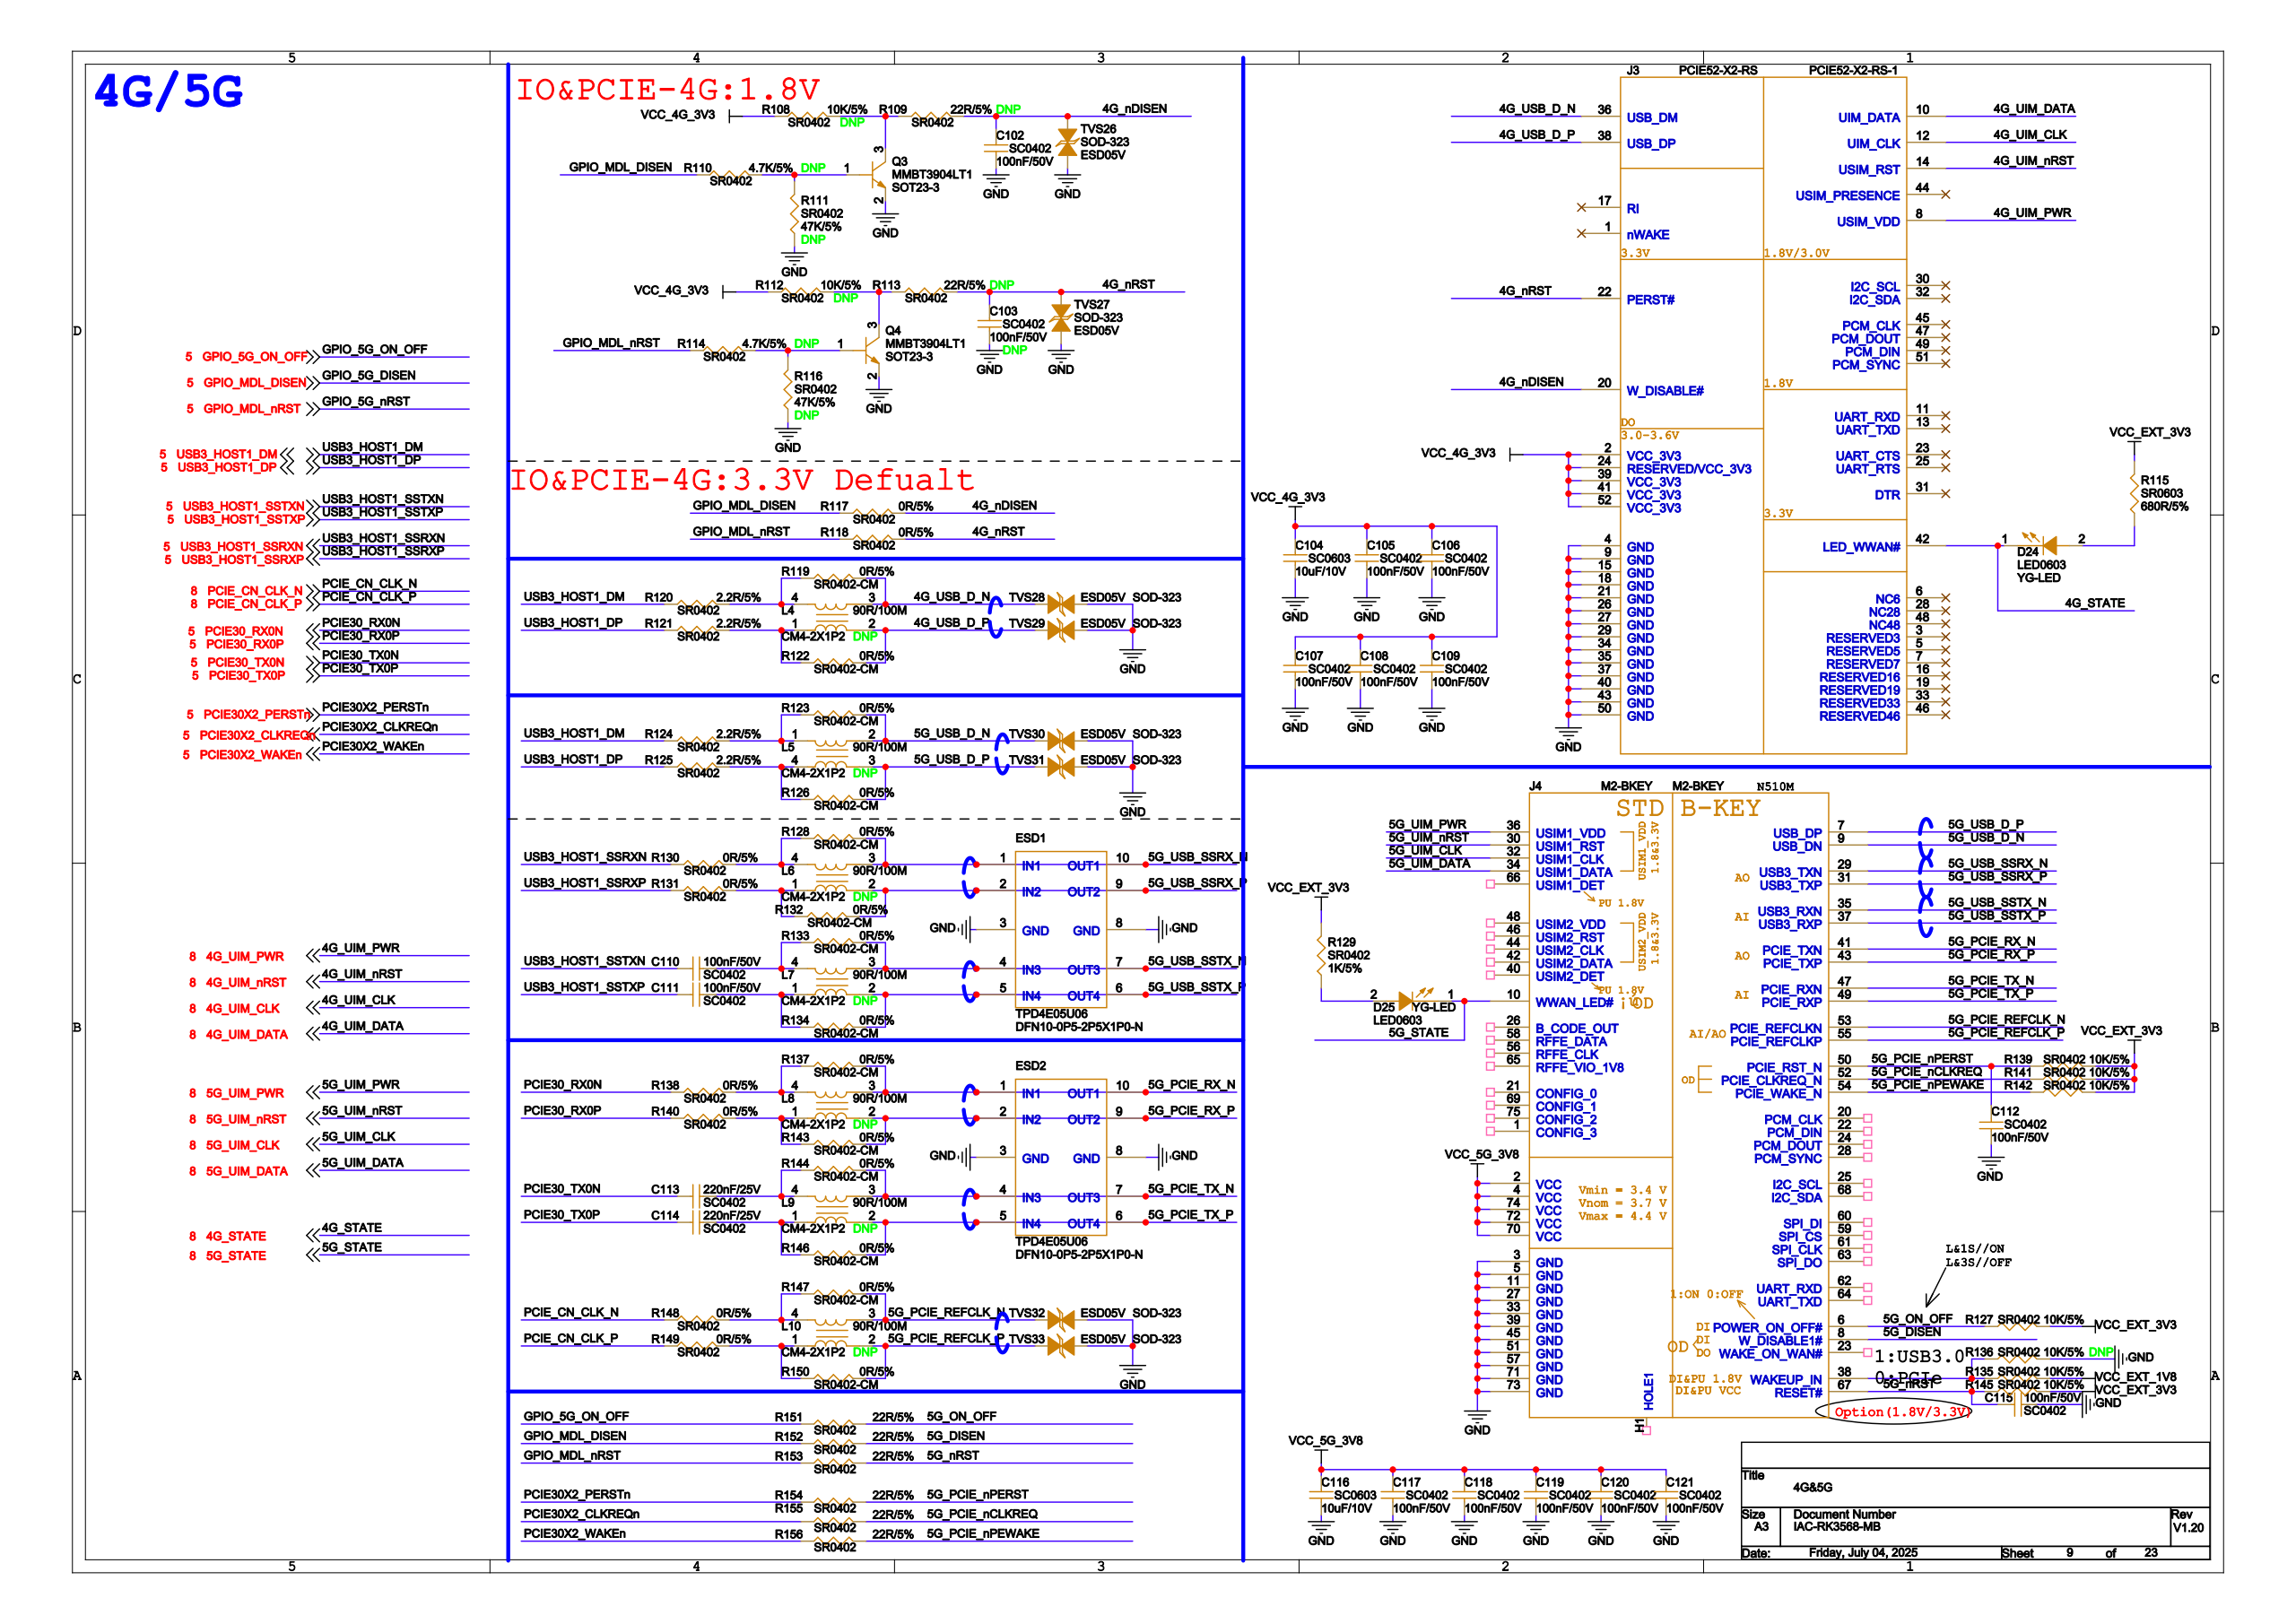Circuit board | Cadence Allegro | 1138 parts | 722 nets | one sheet of the schematic
Parts on this sheet (reference | value | footprint):
C102 | 100nF/50V | SC0402
C103 | 100nF/50V | SC0402
C104 | 10uF/10V | SC0603
C105 | 100nF/50V | SC0402
C106 | 100nF/50V | SC0402
C107 | 100nF/50V | SC0402
C108 | 100nF/50V | SC0402
C109 | 100nF/50V | SC0402
C110 | 100nF/50V | SC0402
C111 | 100nF/50V | SC0402
C112 | 100nF/50V | SC0402
C113 | 220nF/25V | SC0402
C114 | 220nF/25V | SC0402
C115 | 100nF/50V | SC0402
C116 | 10uF/10V | SC0603
C117 | 100nF/50V | SC0402
C118 | 100nF/50V | SC0402
C119 | 100nF/50V | SC0402
C120 | 100nF/50V | SC0402
C121 | 100nF/50V | SC0402
D24 | YG-LED | LED0603
D25 | YG-LED | LED0603
ESD1 | TPD4E05U06 | DFN10-0P5-2P5X1P0-N
ESD2 | TPD4E05U06 | DFN10-0P5-2P5X1P0-N
J3 | PCIE52-X2-RS | PCIE52-X2-RS-1
J4 | M2-BKEY | M2-BKEY
L4 | 90R/100M | CM4-2X1P2
L5 | 90R/100M | CM4-2X1P2
L6 | 90R/100M | CM4-2X1P2
L7 | 90R/100M | CM4-2X1P2
L8 | 90R/100M | CM4-2X1P2
L9 | 90R/100M | CM4-2X1P2
L10 | 90R/100M | CM4-2X1P2
Q3 | MMBT3904LT1 | SOT23-3
Q4 | MMBT3904LT1 | SOT23-3
R108 | 10K/5% | SR0402
R109 | 22R/5% | SR0402
R110 | 4.7K/5% | SR0402
R111 | 47K/5% | SR0402
R112 | 10K/5% | SR0402
R113 | 22R/5% | SR0402
R114 | 4.7K/5% | SR0402
R115 | 680R/5% | SR0603
R116 | 47K/5% | SR0402
R117 | 0R/5% | SR0402
R118 | 0R/5% | SR0402
R119 | 0R/5% | SR0402-CM
R120 | 2.2R/5% | SR0402
R121 | 2.2R/5% | SR0402
R122 | 0R/5% | SR0402-CM
R123 | 0R/5% | SR0402-CM
R124 | 2.2R/5% | SR0402
R125 | 2.2R/5% | SR0402
R126 | 0R/5% | SR0402-CM
R127 | 10K/5% | SR0402
R128 | 0R/5% | SR0402-CM
R129 | 1K/5% | SR0402
R130 | 0R/5% | SR0402
R131 | 0R/5% | SR0402
R132 | 0R/5% | SR0402-CM
R133 | 0R/5% | SR0402-CM
R134 | 0R/5% | SR0402-CM
R135 | 10K/5% | SR0402
R136 | 10K/5% | SR0402
R137 | 0R/5% | SR0402-CM
R138 | 0R/5% | SR0402
R139 | 10K/5% | SR0402
R140 | 0R/5% | SR0402
R141 | 10K/5% | SR0402
R142 | 10K/5% | SR0402
R143 | 0R/5% | SR0402-CM
R144 | 0R/5% | SR0402-CM
R145 | 10K/5% | SR0402
R146 | 0R/5% | SR0402-CM
R147 | 0R/5% | SR0402-CM
R148 | 0R/5% | SR0402
R149 | 0R/5% | SR0402
R150 | 0R/5% | SR0402-CM
R151 | 22R/5% | SR0402
R152 | 22R/5% | SR0402
R153 | 22R/5% | SR0402
R154 | 22R/5% | SR0402
R155 | 22R/5% | SR0402
R156 | 22R/5% | SR0402
TVS26 | ESD05V | SOD-323
TVS27 | ESD05V | SOD-323
TVS28 | ESD05V | SOD-323
TVS29 | ESD05V | SOD-323
TVS30 | ESD05V | SOD-323
TVS31 | ESD05V | SOD-323
TVS32 | ESD05V | SOD-323
TVS33 | ESD05V | SOD-323
Nets of these parts (net: part-pin ...):
VCC_EXT_3V3: R115-2 R127-1 R129-2 R139-1 R141-1 R142-1 R145-2
GND: C102-2 C103-2 C104-2 C105-2 C106-2 C107-2 C108-2 C109-2 C112-1 C115-1 C116-2 C117-2 C118-2 C119-2 C120-2 C121-2 ESD1-3 ESD1-8 ESD2-3 ESD2-8 Q3-2 Q4-2 R111-1 R116-1 R136-1 TVS26-2 TVS27-2 TVS28-1 TVS29-1 TVS30-1 TVS31-1 TVS32-1 TVS33-1 J3-4 J3-9 J3-15 J3-18 J3-21 J3-26 J3-27 J3-29 J3-34 J3-35 J3-37 J3-40 J3-43 J3-50 J4-3 J4-5 J4-11 J4-27 J4-33 J4-39 J4-45 J4-51 J4-57 J4-71 J4-73
4G_NDISEN: C102-1 R109-2 R117-2 TVS26-1 J3-20
4G_NRST: C103-1 R113-2 R118-2 TVS27-1 J3-22
4G_USB_D_N: L4-3 R119-2 TVS28-2 J3-36
4G_USB_D_P: L4-2 R122-2 TVS29-2 J3-38
5G_USB_D_N: L5-2 R123-2 TVS30-2 J4-9
5G_USB_D_P: L5-3 R126-2 TVS31-2 J4-7
5G_PCIE_REFCLK_N: L10-3 R147-2 TVS32-2 J4-53
5G_PCIE_REFCLK_P: L10-2 R150-2 TVS33-2 J4-55
4G_STATE: D24-1 J3-42
VCC_4G_3V3: C104-1 C105-1 C106-1 C107-1 C108-1 C109-1 R108-1 R112-1 J3-2 J3-24 J3-39 J3-41 J3-52
4G_UIM_CLK: J3-12 J4-32
4G_UIM_DATA: J3-10 J4-34
4G_UIM_PWR: J3-8 J4-36
N4026883: L4-4 R119-1 R120-2
N4026879: L4-1 R121-2 R122-1
N4049312: L5-1 R123-1 R124-2
N4049308: L5-4 R125-2 R126-1
N4049390: L6-4 R128-1 R130-2
5G_USB_SSRX_N: ESD1-1 ESD1-10 L6-3 R128-2 J4-29
N4049436: L6-1 R131-2 R132-1
5G_USB_SSRX_P: ESD1-2 ESD1-9 L6-2 R132-2 J4-31
N4049484: C110-2 L7-4 R133-1
5G_USB_SSTX_N: ESD1-4 ESD1-7 L7-3 R133-2 J4-35
N4049500: C111-2 L7-1 R134-1
5G_USB_SSTX_P: ESD1-5 ESD1-6 L7-2 R134-2 J4-37
N4049040: L8-4 R137-1 R138-2
5G_PCIE_RX_N: ESD2-1 ESD2-10 L8-3 R137-2 J4-41
N4049036: L8-1 R140-2 R143-1
5G_PCIE_RX_P: ESD2-2 ESD2-9 L8-2 R143-2 J4-43
N4048764: C113-2 L9-4 R144-1
5G_PCIE_TX_N: ESD2-4 ESD2-7 L9-3 R144-2 J4-47
N4048740: C114-2 L9-1 R146-1
5G_PCIE_TX_P: ESD2-5 ESD2-6 L9-2 R146-2 J4-49
N4049060: L10-4 R147-1 R148-2
N4049056: L10-1 R149-2 R150-1
5G_PCIE_NCLKREQ: R141-2 R155-2 J4-52
5G_PCIE_NPERST: C112-2 R139-2 R154-2 J4-50
5G_PCIE_NPEWAKE: R142-2 R156-2 J4-54
5G_ON_OFF: R127-2 R151-2 J4-6
5G_NRST: C115-2 R145-1 R153-2 J4-67
VCC_5G_3V8: C116-1 C117-1 C118-1 C119-1 C120-1 C121-1 J4-2 J4-4 J4-70 J4-72 J4-74
N4020192: R135-2 R136-2 J4-38
5G_STATE: D25-1 J4-10
5G_DISEN: R152-2 J4-8
VCC_EXT_1V8: R135-1
N4026257: Q3-1 R110-2 R111-2
N4026253: Q3-3 R108-2 R109-1
N4026425: Q4-1 R114-2 R116-2
N4026421: Q4-3 R112-2 R113-1
PCIE30_TX0N: C113-1
PCIE30_TX0P: C114-1
N4027963: D24-2 R115-1
N4020438: D25-2 R129-1
PCIE_CN_CLK_P: R149-1
PCIE_CN_CLK_N: R148-1
USB3_HOST1_DM: R120-1 R124-1
USB3_HOST1_DP: R121-1 R125-1
GPIO_MDL_DISEN: R110-1 R117-1 R152-1
GPIO_MDL_NRST: R114-1 R118-1 R153-1
PCIE30X2_CLKREQN: R155-1
PCIE30X2_WAKEN: R156-1
PCIE30X2_PERSTN: R154-1
GPIO_5G_ON_OFF: R151-1
PCIE30_RX0N: R138-1
PCIE30_RX0P: R140-1
USB3_HOST1_SSRXN: R130-1
USB3_HOST1_SSRXP: R131-1
USB3_HOST1_SSTXN: C110-1
USB3_HOST1_SSTXP: C111-1